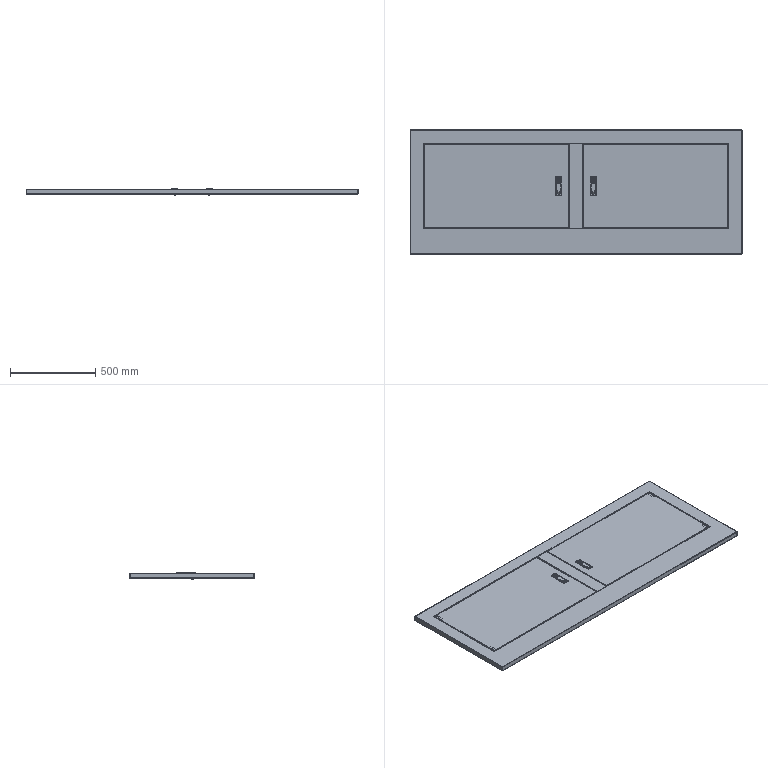Part | SolidWorks | features MirrorCompFeat 1, ReferencePattern 1 | 14 solids | 1028 faces | box 1950 x 730 x 42.5 mm | volume 3302134 mm3 | plane 580 | cylinder 336 | spline 88 | cone 24 | commonest cylinder face diameters 4 x88 1 x54 2 x30 5 x16 12 x16 8 x12